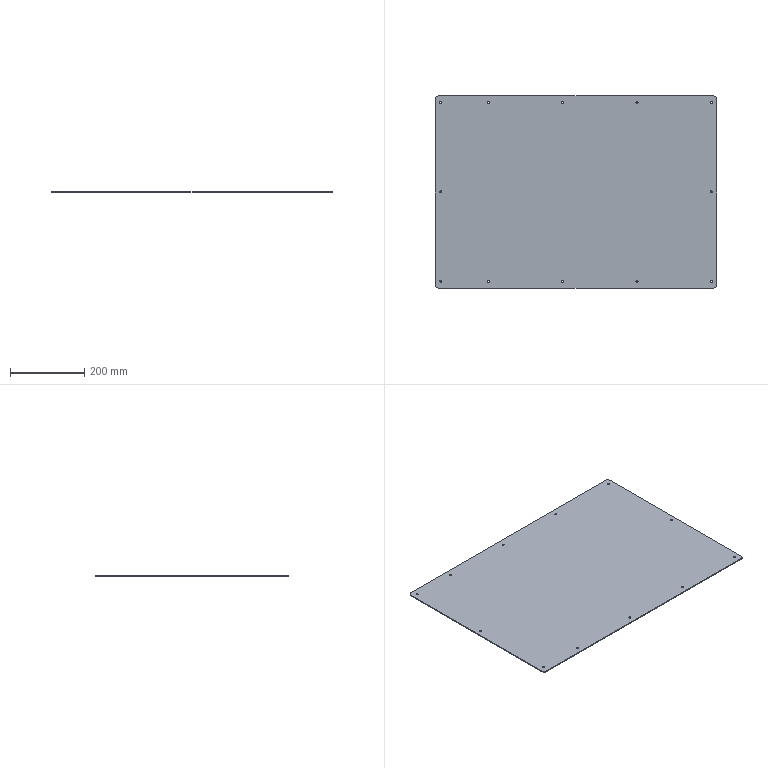Part | STEP file | MT-COMBO-119-S008 | 1 solid | 34 faces | box 758 x 516.5 x 2.5 mm | volume 977840 mm3 | cylinder 28 | plane 6 | commonest cylinder face diameters 5.5 x24 20 x4
STEP:
#1=CARTESIAN_POINT('',(-33.25,240.25,2.5));
#2=VERTEX_POINT('',#1);
#3=CARTESIAN_POINT('',(-38.75,240.25,2.5));
#4=VERTEX_POINT('',#3);
#5=CARTESIAN_POINT('',(-36.,240.25,2.5));
#6=DIRECTION('',(0.,0.,-1.));
#7=DIRECTION('',(-1.,0.,0.));
#8=AXIS2_PLACEMENT_3D('',#5,#6,#7);
#9=CIRCLE('',#8,2.75);
#10=EDGE_CURVE('',#2,#4,#9,.T.);
#11=ORIENTED_EDGE('',*,*,#10,.F.);
#12=CARTESIAN_POINT('',(-33.25,240.25,0.));
#13=VERTEX_POINT('',#12);
#14=CARTESIAN_POINT('',(-33.25,240.25,0.));
#15=DIRECTION('',(0.,0.,-1.));
#16=VECTOR('',#15,1000.);
#17=LINE('',#14,#16);
#18=EDGE_CURVE('',#2,#13,#17,.T.);
#19=ORIENTED_EDGE('',*,*,#18,.T.);
#20=CARTESIAN_POINT('',(-38.75,240.25,0.));
#21=VERTEX_POINT('',#20);
#22=CARTESIAN_POINT('',(-36.,240.25,0.));
#23=DIRECTION('',(0.,0.,-1.));
#24=DIRECTION('',(-1.,0.,0.));
#25=AXIS2_PLACEMENT_3D('',#22,#23,#24);
#26=CIRCLE('',#25,2.75);
#27=EDGE_CURVE('',#13,#21,#26,.T.);
#28=ORIENTED_EDGE('',*,*,#27,.T.);
#29=CARTESIAN_POINT('',(-38.75,240.25,0.));
#30=DIRECTION('',(0.,0.,-1.));
#31=VECTOR('',#30,1000.);
#32=LINE('',#29,#31);
#33=EDGE_CURVE('',#4,#21,#32,.T.);
#34=ORIENTED_EDGE('',*,*,#33,.F.);
#35=EDGE_LOOP('',(#11,#19,#28,#34));
#36=FACE_OUTER_BOUND('',#35,.T.);
#37=CARTESIAN_POINT('',(-36.,240.25,0.));
#38=DIRECTION('',(0.,0.,-1.));
#39=DIRECTION('',(-1.,0.,0.));
#40=AXIS2_PLACEMENT_3D('',#37,#38,#39);
#41=CYLINDRICAL_SURFACE('',#40,2.75);
#42=ADVANCED_FACE('',(#36),#41,.F.);
#43=CARTESIAN_POINT('',(-233.25,-240.25,2.5));
#44=VERTEX_POINT('',#43);
#45=CARTESIAN_POINT('',(-238.75,-240.25,2.5));
#46=VERTEX_POINT('',#45);
#47=CARTESIAN_POINT('',(-236.,-240.25,2.5));
#48=DIRECTION('',(0.,0.,-1.));
#49=DIRECTION('',(-1.,0.,0.));
#50=AXIS2_PLACEMENT_3D('',#47,#48,#49);
#51=CIRCLE('',#50,2.75);
#52=EDGE_CURVE('',#44,#46,#51,.T.);
#53=ORIENTED_EDGE('',*,*,#52,.F.);
#54=CARTESIAN_POINT('',(-233.25,-240.25,0.));
#55=VERTEX_POINT('',#54);
#56=CARTESIAN_POINT('',(-233.25,-240.25,0.));
#57=DIRECTION('',(0.,0.,-1.));
#58=VECTOR('',#57,1000.);
#59=LINE('',#56,#58);
#60=EDGE_CURVE('',#44,#55,#59,.T.);
#61=ORIENTED_EDGE('',*,*,#60,.T.);
#62=CARTESIAN_POINT('',(-238.75,-240.25,0.));
#63=VERTEX_POINT('',#62);
#64=CARTESIAN_POINT('',(-236.,-240.25,0.));
#65=DIRECTION('',(0.,0.,-1.));
#66=DIRECTION('',(-1.,0.,0.));
#67=AXIS2_PLACEMENT_3D('',#64,#65,#66);
#68=CIRCLE('',#67,2.75);
#69=EDGE_CURVE('',#55,#63,#68,.T.);
#70=ORIENTED_EDGE('',*,*,#69,.T.);
#71=CARTESIAN_POINT('',(-238.75,-240.25,0.));
#72=DIRECTION('',(0.,0.,-1.));
#73=VECTOR('',#72,1000.);
#74=LINE('',#71,#73);
#75=EDGE_CURVE('',#46,#63,#74,.T.);
#76=ORIENTED_EDGE('',*,*,#75,.F.);
#77=EDGE_LOOP('',(#53,#61,#70,#76));
#78=FACE_OUTER_BOUND('',#77,.T.);
#79=CARTESIAN_POINT('',(-236.,-240.25,0.));
#80=DIRECTION('',(0.,0.,-1.));
#81=DIRECTION('',(-1.,0.,0.));
#82=AXIS2_PLACEMENT_3D('',#79,#80,#81);
#83=CYLINDRICAL_SURFACE('',#82,2.75);
#84=ADVANCED_FACE('',(#78),#83,.F.);
#85=CARTESIAN_POINT('',(-33.25,-240.25,2.5));
#86=VERTEX_POINT('',#85);
#87=CARTESIAN_POINT('',(-38.75,-240.25,2.5));
#88=VERTEX_POINT('',#87);
#89=CARTESIAN_POINT('',(-36.,-240.25,2.5));
#90=DIRECTION('',(0.,0.,-1.));
#91=DIRECTION('',(-1.,0.,0.));
#92=AXIS2_PLACEMENT_3D('',#89,#90,#91);
#93=CIRCLE('',#92,2.75);
#94=EDGE_CURVE('',#86,#88,#93,.T.);
#95=ORIENTED_EDGE('',*,*,#94,.F.);
#96=CARTESIAN_POINT('',(-33.25,-240.25,0.));
#97=VERTEX_POINT('',#96);
#98=CARTESIAN_POINT('',(-33.25,-240.25,0.));
#99=DIRECTION('',(0.,0.,-1.));
#100=VECTOR('',#99,1000.);
#101=LINE('',#98,#100);
#102=EDGE_CURVE('',#86,#97,#101,.T.);
#103=ORIENTED_EDGE('',*,*,#102,.T.);
#104=CARTESIAN_POINT('',(-38.75,-240.25,0.));
#105=VERTEX_POINT('',#104);
#106=CARTESIAN_POINT('',(-36.,-240.25,0.));
#107=DIRECTION('',(0.,0.,-1.));
#108=DIRECTION('',(-1.,0.,0.));
#109=AXIS2_PLACEMENT_3D('',#106,#107,#108);
#110=CIRCLE('',#109,2.75);
#111=EDGE_CURVE('',#97,#105,#110,.T.);
#112=ORIENTED_EDGE('',*,*,#111,.T.);
#113=CARTESIAN_POINT('',(-38.75,-240.25,0.));
#114=DIRECTION('',(0.,0.,-1.));
#115=VECTOR('',#114,1000.);
#116=LINE('',#113,#115);
#117=EDGE_CURVE('',#88,#105,#116,.T.);
#118=ORIENTED_EDGE('',*,*,#117,.F.);
#119=EDGE_LOOP('',(#95,#103,#112,#118));
#120=FACE_OUTER_BOUND('',#119,.T.);
#121=CARTESIAN_POINT('',(-36.,-240.25,0.));
#122=DIRECTION('',(0.,0.,-1.));
#123=DIRECTION('',(-1.,0.,0.));
#124=AXIS2_PLACEMENT_3D('',#121,#122,#123);
#125=CYLINDRICAL_SURFACE('',#124,2.75);
#126=ADVANCED_FACE('',(#120),#125,.F.);
#127=CARTESIAN_POINT('',(166.75,-240.25,2.5));
#128=VERTEX_POINT('',#127);
#129=CARTESIAN_POINT('',(161.25,-240.25,2.5));
#130=VERTEX_POINT('',#129);
#131=CARTESIAN_POINT('',(164.,-240.25,2.5));
#132=DIRECTION('',(0.,0.,-1.));
#133=DIRECTION('',(-1.,0.,0.));
#134=AXIS2_PLACEMENT_3D('',#131,#132,#133);
#135=CIRCLE('',#134,2.75);
#136=EDGE_CURVE('',#128,#130,#135,.T.);
#137=ORIENTED_EDGE('',*,*,#136,.F.);
#138=CARTESIAN_POINT('',(166.75,-240.25,0.));
#139=VERTEX_POINT('',#138);
#140=CARTESIAN_POINT('',(166.75,-240.25,0.));
#141=DIRECTION('',(0.,0.,-1.));
#142=VECTOR('',#141,1000.);
#143=LINE('',#140,#142);
#144=EDGE_CURVE('',#128,#139,#143,.T.);
#145=ORIENTED_EDGE('',*,*,#144,.T.);
#146=CARTESIAN_POINT('',(161.25,-240.25,0.));
#147=VERTEX_POINT('',#146);
#148=CARTESIAN_POINT('',(164.,-240.25,0.));
#149=DIRECTION('',(0.,0.,-1.));
#150=DIRECTION('',(-1.,0.,0.));
#151=AXIS2_PLACEMENT_3D('',#148,#149,#150);
#152=CIRCLE('',#151,2.75);
#153=EDGE_CURVE('',#139,#147,#152,.T.);
#154=ORIENTED_EDGE('',*,*,#153,.T.);
#155=CARTESIAN_POINT('',(161.25,-240.25,0.));
#156=DIRECTION('',(0.,0.,-1.));
#157=VECTOR('',#156,1000.);
#158=LINE('',#155,#157);
#159=EDGE_CURVE('',#130,#147,#158,.T.);
#160=ORIENTED_EDGE('',*,*,#159,.F.);
#161=EDGE_LOOP('',(#137,#145,#154,#160));
#162=FACE_OUTER_BOUND('',#161,.T.);
#163=CARTESIAN_POINT('',(164.,-240.25,0.));
#164=DIRECTION('',(0.,0.,-1.));
#165=DIRECTION('',(-1.,0.,0.));
#166=AXIS2_PLACEMENT_3D('',#163,#164,#165);
#167=CYLINDRICAL_SURFACE('',#166,2.75);
#168=ADVANCED_FACE('',(#162),#167,.F.);
#169=CARTESIAN_POINT('',(366.75,240.25,2.5));
#170=VERTEX_POINT('',#169);
#171=CARTESIAN_POINT('',(361.25,240.25,2.5));
#172=VERTEX_POINT('',#171);
#173=CARTESIAN_POINT('',(364.,240.25,2.5));
#174=DIRECTION('',(0.,0.,-1.));
#175=DIRECTION('',(-1.,0.,0.));
#176=AXIS2_PLACEMENT_3D('',#173,#174,#175);
#177=CIRCLE('',#176,2.75);
#178=EDGE_CURVE('',#170,#172,#177,.T.);
#179=ORIENTED_EDGE('',*,*,#178,.F.);
#180=CARTESIAN_POINT('',(366.75,240.25,0.));
#181=VERTEX_POINT('',#180);
#182=CARTESIAN_POINT('',(366.75,240.25,0.));
#183=DIRECTION('',(0.,0.,-1.));
#184=VECTOR('',#183,1000.);
#185=LINE('',#182,#184);
#186=EDGE_CURVE('',#170,#181,#185,.T.);
#187=ORIENTED_EDGE('',*,*,#186,.T.);
#188=CARTESIAN_POINT('',(361.25,240.25,0.));
#189=VERTEX_POINT('',#188);
#190=CARTESIAN_POINT('',(364.,240.25,0.));
#191=DIRECTION('',(0.,0.,-1.));
#192=DIRECTION('',(-1.,0.,0.));
#193=AXIS2_PLACEMENT_3D('',#190,#191,#192);
#194=CIRCLE('',#193,2.75);
#195=EDGE_CURVE('',#181,#189,#194,.T.);
#196=ORIENTED_EDGE('',*,*,#195,.T.);
#197=CARTESIAN_POINT('',(361.25,240.25,0.));
#198=DIRECTION('',(0.,0.,-1.));
#199=VECTOR('',#198,1000.);
#200=LINE('',#197,#199);
#201=EDGE_CURVE('',#172,#189,#200,.T.);
#202=ORIENTED_EDGE('',*,*,#201,.F.);
#203=EDGE_LOOP('',(#179,#187,#196,#202));
#204=FACE_OUTER_BOUND('',#203,.T.);
#205=CARTESIAN_POINT('',(364.,240.25,0.));
#206=DIRECTION('',(0.,0.,-1.));
#207=DIRECTION('',(-1.,0.,0.));
#208=AXIS2_PLACEMENT_3D('',#205,#206,#207);
#209=CYLINDRICAL_SURFACE('',#208,2.75);
#210=ADVANCED_FACE('',(#204),#209,.F.);
#211=CARTESIAN_POINT('',(366.75,-240.25,2.5));
#212=VERTEX_POINT('',#211);
#213=CARTESIAN_POINT('',(361.25,-240.25,2.5));
#214=VERTEX_POINT('',#213);
#215=CARTESIAN_POINT('',(364.,-240.25,2.5));
#216=DIRECTION('',(0.,0.,-1.));
#217=DIRECTION('',(-1.,0.,0.));
#218=AXIS2_PLACEMENT_3D('',#215,#216,#217);
#219=CIRCLE('',#218,2.75);
#220=EDGE_CURVE('',#212,#214,#219,.T.);
#221=ORIENTED_EDGE('',*,*,#220,.F.);
#222=CARTESIAN_POINT('',(366.75,-240.25,0.));
#223=VERTEX_POINT('',#222);
#224=CARTESIAN_POINT('',(366.75,-240.25,0.));
#225=DIRECTION('',(0.,0.,-1.));
#226=VECTOR('',#225,1000.);
#227=LINE('',#224,#226);
#228=EDGE_CURVE('',#212,#223,#227,.T.);
#229=ORIENTED_EDGE('',*,*,#228,.T.);
#230=CARTESIAN_POINT('',(361.25,-240.25,0.));
#231=VERTEX_POINT('',#230);
#232=CARTESIAN_POINT('',(364.,-240.25,0.));
#233=DIRECTION('',(0.,0.,-1.));
#234=DIRECTION('',(-1.,0.,0.));
#235=AXIS2_PLACEMENT_3D('',#232,#233,#234);
#236=CIRCLE('',#235,2.75);
#237=EDGE_CURVE('',#223,#231,#236,.T.);
#238=ORIENTED_EDGE('',*,*,#237,.T.);
#239=CARTESIAN_POINT('',(361.25,-240.25,0.));
#240=DIRECTION('',(0.,0.,-1.));
#241=VECTOR('',#240,1000.);
#242=LINE('',#239,#241);
#243=EDGE_CURVE('',#214,#231,#242,.T.);
#244=ORIENTED_EDGE('',*,*,#243,.F.);
#245=EDGE_LOOP('',(#221,#229,#238,#244));
#246=FACE_OUTER_BOUND('',#245,.T.);
#247=CARTESIAN_POINT('',(364.,-240.25,0.));
#248=DIRECTION('',(0.,0.,-1.));
#249=DIRECTION('',(-1.,0.,0.));
#250=AXIS2_PLACEMENT_3D('',#247,#248,#249);
#251=CYLINDRICAL_SURFACE('',#250,2.75);
#252=ADVANCED_FACE('',(#246),#251,.F.);
#253=CARTESIAN_POINT('',(366.75,0.25,2.5));
#254=VERTEX_POINT('',#253);
#255=CARTESIAN_POINT('',(361.25,0.25,2.5));
#256=VERTEX_POINT('',#255);
#257=CARTESIAN_POINT('',(364.,0.25,2.5));
#258=DIRECTION('',(0.,0.,-1.));
#259=DIRECTION('',(-1.,0.,0.));
#260=AXIS2_PLACEMENT_3D('',#257,#258,#259);
#261=CIRCLE('',#260,2.75);
#262=EDGE_CURVE('',#254,#256,#261,.T.);
#263=ORIENTED_EDGE('',*,*,#262,.F.);
#264=CARTESIAN_POINT('',(366.75,0.25,0.));
#265=VERTEX_POINT('',#264);
#266=CARTESIAN_POINT('',(366.75,0.25,0.));
#267=DIRECTION('',(0.,0.,-1.));
#268=VECTOR('',#267,1000.);
#269=LINE('',#266,#268);
#270=EDGE_CURVE('',#254,#265,#269,.T.);
#271=ORIENTED_EDGE('',*,*,#270,.T.);
#272=CARTESIAN_POINT('',(361.25,0.25,0.));
#273=VERTEX_POINT('',#272);
#274=CARTESIAN_POINT('',(364.,0.25,0.));
#275=DIRECTION('',(0.,0.,-1.));
#276=DIRECTION('',(-1.,0.,0.));
#277=AXIS2_PLACEMENT_3D('',#274,#275,#276);
#278=CIRCLE('',#277,2.75);
#279=EDGE_CURVE('',#265,#273,#278,.T.);
#280=ORIENTED_EDGE('',*,*,#279,.T.);
#281=CARTESIAN_POINT('',(361.25,0.25,0.));
#282=DIRECTION('',(0.,0.,-1.));
#283=VECTOR('',#282,1000.);
#284=LINE('',#281,#283);
#285=EDGE_CURVE('',#256,#273,#284,.T.);
#286=ORIENTED_EDGE('',*,*,#285,.F.);
#287=EDGE_LOOP('',(#263,#271,#280,#286));
#288=FACE_OUTER_BOUND('',#287,.T.);
#289=CARTESIAN_POINT('',(364.,0.25,0.));
#290=DIRECTION('',(0.,0.,-1.));
#291=DIRECTION('',(-1.,0.,0.));
#292=AXIS2_PLACEMENT_3D('',#289,#290,#291);
#293=CYLINDRICAL_SURFACE('',#292,2.75);
#294=ADVANCED_FACE('',(#288),#293,.F.);
#295=CARTESIAN_POINT('',(-361.25,240.25,2.5));
#296=VERTEX_POINT('',#295);
#297=CARTESIAN_POINT('',(-366.75,240.25,2.5));
#298=VERTEX_POINT('',#297);
#299=CARTESIAN_POINT('',(-364.,240.25,2.5));
#300=DIRECTION('',(0.,0.,-1.));
#301=DIRECTION('',(-1.,0.,0.));
#302=AXIS2_PLACEMENT_3D('',#299,#300,#301);
#303=CIRCLE('',#302,2.75);
#304=EDGE_CURVE('',#296,#298,#303,.T.);
#305=ORIENTED_EDGE('',*,*,#304,.F.);
#306=CARTESIAN_POINT('',(-361.25,240.25,0.));
#307=VERTEX_POINT('',#306);
#308=CARTESIAN_POINT('',(-361.25,240.25,0.));
#309=DIRECTION('',(0.,0.,-1.));
#310=VECTOR('',#309,1000.);
#311=LINE('',#308,#310);
#312=EDGE_CURVE('',#296,#307,#311,.T.);
#313=ORIENTED_EDGE('',*,*,#312,.T.);
#314=CARTESIAN_POINT('',(-366.75,240.25,0.));
#315=VERTEX_POINT('',#314);
#316=CARTESIAN_POINT('',(-364.,240.25,0.));
#317=DIRECTION('',(0.,0.,-1.));
#318=DIRECTION('',(-1.,0.,0.));
#319=AXIS2_PLACEMENT_3D('',#316,#317,#318);
#320=CIRCLE('',#319,2.75);
#321=EDGE_CURVE('',#307,#315,#320,.T.);
#322=ORIENTED_EDGE('',*,*,#321,.T.);
#323=CARTESIAN_POINT('',(-366.75,240.25,0.));
#324=DIRECTION('',(0.,0.,-1.));
#325=VECTOR('',#324,1000.);
#326=LINE('',#323,#325);
#327=EDGE_CURVE('',#298,#315,#326,.T.);
#328=ORIENTED_EDGE('',*,*,#327,.F.);
#329=EDGE_LOOP('',(#305,#313,#322,#328));
#330=FACE_OUTER_BOUND('',#329,.T.);
#331=CARTESIAN_POINT('',(-364.,240.25,0.));
#332=DIRECTION('',(0.,0.,-1.));
#333=DIRECTION('',(-1.,0.,0.));
#334=AXIS2_PLACEMENT_3D('',#331,#332,#333);
#335=CYLINDRICAL_SURFACE('',#334,2.75);
#336=ADVANCED_FACE('',(#330),#335,.F.);
#337=CARTESIAN_POINT('',(-361.25,-239.75,2.5));
#338=VERTEX_POINT('',#337);
#339=CARTESIAN_POINT('',(-366.75,-239.75,2.5));
#340=VERTEX_POINT('',#339);
#341=CARTESIAN_POINT('',(-364.,-239.75,2.5));
#342=DIRECTION('',(0.,0.,-1.));
#343=DIRECTION('',(-1.,0.,0.));
#344=AXIS2_PLACEMENT_3D('',#341,#342,#343);
#345=CIRCLE('',#344,2.75);
#346=EDGE_CURVE('',#338,#340,#345,.T.);
#347=ORIENTED_EDGE('',*,*,#346,.F.);
#348=CARTESIAN_POINT('',(-361.25,-239.75,0.));
#349=VERTEX_POINT('',#348);
#350=CARTESIAN_POINT('',(-361.25,-239.75,0.));
#351=DIRECTION('',(0.,0.,-1.));
#352=VECTOR('',#351,1000.);
#353=LINE('',#350,#352);
#354=EDGE_CURVE('',#338,#349,#353,.T.);
#355=ORIENTED_EDGE('',*,*,#354,.T.);
#356=CARTESIAN_POINT('',(-366.75,-239.75,0.));
#357=VERTEX_POINT('',#356);
#358=CARTESIAN_POINT('',(-364.,-239.75,0.));
#359=DIRECTION('',(0.,0.,-1.));
#360=DIRECTION('',(-1.,0.,0.));
#361=AXIS2_PLACEMENT_3D('',#358,#359,#360);
#362=CIRCLE('',#361,2.75);
#363=EDGE_CURVE('',#349,#357,#362,.T.);
#364=ORIENTED_EDGE('',*,*,#363,.T.);
#365=CARTESIAN_POINT('',(-366.75,-239.75,0.));
#366=DIRECTION('',(0.,0.,-1.));
#367=VECTOR('',#366,1000.);
#368=LINE('',#365,#367);
#369=EDGE_CURVE('',#340,#357,#368,.T.);
#370=ORIENTED_EDGE('',*,*,#369,.F.);
#371=EDGE_LOOP('',(#347,#355,#364,#370));
#372=FACE_OUTER_BOUND('',#371,.T.);
#373=CARTESIAN_POINT('',(-364.,-239.75,0.));
#374=DIRECTION('',(0.,0.,-1.));
#375=DIRECTION('',(-1.,0.,0.));
#376=AXIS2_PLACEMENT_3D('',#373,#374,#375);
#377=CYLINDRICAL_SURFACE('',#376,2.75);
#378=ADVANCED_FACE('',(#372),#377,.F.);
#379=CARTESIAN_POINT('',(-361.25,0.25,2.5));
#380=VERTEX_POINT('',#379);
#381=CARTESIAN_POINT('',(-366.75,0.25,2.5));
#382=VERTEX_POINT('',#381);
#383=CARTESIAN_POINT('',(-364.,0.25,2.5));
#384=DIRECTION('',(0.,0.,-1.));
#385=DIRECTION('',(-1.,0.,0.));
#386=AXIS2_PLACEMENT_3D('',#383,#384,#385);
#387=CIRCLE('',#386,2.75);
#388=EDGE_CURVE('',#380,#382,#387,.T.);
#389=ORIENTED_EDGE('',*,*,#388,.F.);
#390=CARTESIAN_POINT('',(-361.25,0.25,0.));
#391=VERTEX_POINT('',#390);
#392=CARTESIAN_POINT('',(-361.25,0.25,0.));
#393=DIRECTION('',(0.,0.,-1.));
#394=VECTOR('',#393,1000.);
#395=LINE('',#392,#394);
#396=EDGE_CURVE('',#380,#391,#395,.T.);
#397=ORIENTED_EDGE('',*,*,#396,.T.);
#398=CARTESIAN_POINT('',(-366.75,0.25,0.));
#399=VERTEX_POINT('',#398);
#400=CARTESIAN_POINT('',(-364.,0.25,0.));
#401=DIRECTION('',(0.,0.,-1.));
#402=DIRECTION('',(-1.,0.,0.));
#403=AXIS2_PLACEMENT_3D('',#400,#401,#402);
#404=CIRCLE('',#403,2.75);
#405=EDGE_CURVE('',#391,#399,#404,.T.);
#406=ORIENTED_EDGE('',*,*,#405,.T.);
#407=CARTESIAN_POINT('',(-366.75,0.25,0.));
#408=DIRECTION('',(0.,0.,-1.));
#409=VECTOR('',#408,1000.);
#410=LINE('',#407,#409);
#411=EDGE_CURVE('',#382,#399,#410,.T.);
#412=ORIENTED_EDGE('',*,*,#411,.F.);
#413=EDGE_LOOP('',(#389,#397,#406,#412));
#414=FACE_OUTER_BOUND('',#413,.T.);
#415=CARTESIAN_POINT('',(-364.,0.25,0.));
#416=DIRECTION('',(0.,0.,-1.));
#417=DIRECTION('',(-1.,0.,0.));
#418=AXIS2_PLACEMENT_3D('',#415,#416,#417);
#419=CYLINDRICAL_SURFACE('',#418,2.75);
#420=ADVANCED_FACE('',(#414),#419,.F.);
#421=CARTESIAN_POINT('',(166.75,240.25,2.5));
#422=VERTEX_POINT('',#421);
#423=CARTESIAN_POINT('',(161.25,240.25,2.5));
#424=VERTEX_POINT('',#423);
#425=CARTESIAN_POINT('',(164.,240.25,2.5));
#426=DIRECTION('',(0.,0.,-1.));
#427=DIRECTION('',(-1.,0.,0.));
#428=AXIS2_PLACEMENT_3D('',#425,#426,#427);
#429=CIRCLE('',#428,2.75);
#430=EDGE_CURVE('',#422,#424,#429,.T.);
#431=ORIENTED_EDGE('',*,*,#430,.F.);
#432=CARTESIAN_POINT('',(166.75,240.25,0.));
#433=VERTEX_POINT('',#432);
#434=CARTESIAN_POINT('',(166.75,240.25,0.));
#435=DIRECTION('',(0.,0.,-1.));
#436=VECTOR('',#435,1000.);
#437=LINE('',#434,#436);
#438=EDGE_CURVE('',#422,#433,#437,.T.);
#439=ORIENTED_EDGE('',*,*,#438,.T.);
#440=CARTESIAN_POINT('',(161.25,240.25,0.));
#441=VERTEX_POINT('',#440);
#442=CARTESIAN_POINT('',(164.,240.25,0.));
#443=DIRECTION('',(0.,0.,-1.));
#444=DIRECTION('',(-1.,0.,0.));
#445=AXIS2_PLACEMENT_3D('',#442,#443,#444);
#446=CIRCLE('',#445,2.75);
#447=EDGE_CURVE('',#433,#441,#446,.T.);
#448=ORIENTED_EDGE('',*,*,#447,.T.);
#449=CARTESIAN_POINT('',(161.25,240.25,0.));
#450=DIRECTION('',(0.,0.,-1.));
#451=VECTOR('',#450,1000.);
#452=LINE('',#449,#451);
#453=EDGE_CURVE('',#424,#441,#452,.T.);
#454=ORIENTED_EDGE('',*,*,#453,.F.);
#455=EDGE_LOOP('',(#431,#439,#448,#454));
#456=FACE_OUTER_BOUND('',#455,.T.);
#457=CARTESIAN_POINT('',(164.,240.25,0.));
#458=DIRECTION('',(0.,0.,-1.));
#459=DIRECTION('',(-1.,0.,0.));
#460=AXIS2_PLACEMENT_3D('',#457,#458,#459);
#461=CYLINDRICAL_SURFACE('',#460,2.75);
#462=ADVANCED_FACE('',(#456),#461,.F.);
#463=CARTESIAN_POINT('',(-233.25,240.25,2.5));
#464=VERTEX_POINT('',#463);
#465=CARTESIAN_POINT('',(-238.75,240.25,2.5));
#466=VERTEX_POINT('',#465);
#467=CARTESIAN_POINT('',(-236.,240.25,2.5));
#468=DIRECTION('',(0.,0.,-1.));
#469=DIRECTION('',(-1.,0.,0.));
#470=AXIS2_PLACEMENT_3D('',#467,#468,#469);
#471=CIRCLE('',#470,2.75);
#472=EDGE_CURVE('',#464,#466,#471,.T.);
#473=ORIENTED_EDGE('',*,*,#472,.F.);
#474=CARTESIAN_POINT('',(-233.25,240.25,0.));
#475=VERTEX_POINT('',#474);
#476=CARTESIAN_POINT('',(-233.25,240.25,0.));
#477=DIRECTION('',(0.,0.,-1.));
#478=VECTOR('',#477,1000.);
#479=LINE('',#476,#478);
#480=EDGE_CURVE('',#464,#475,#479,.T.);
#481=ORIENTED_EDGE('',*,*,#480,.T.);
#482=CARTESIAN_POINT('',(-238.75,240.25,0.));
#483=VERTEX_POINT('',#482);
#484=CARTESIAN_POINT('',(-236.,240.25,0.));
#485=DIRECTION('',(0.,0.,-1.));
#486=DIRECTION('',(-1.,0.,0.));
#487=AXIS2_PLACEMENT_3D('',#484,#485,#486);
#488=CIRCLE('',#487,2.75);
#489=EDGE_CURVE('',#475,#483,#488,.T.);
#490=ORIENTED_EDGE('',*,*,#489,.T.);
#491=CARTESIAN_POINT('',(-238.75,240.25,0.));
#492=DIRECTION('',(0.,0.,-1.));
#493=VECTOR('',#492,1000.);
#494=LINE('',#491,#493);
#495=EDGE_CURVE('',#466,#483,#494,.T.);
#496=ORIENTED_EDGE('',*,*,#495,.F.);
#497=EDGE_LOOP('',(#473,#481,#490,#496));
#498=FACE_OUTER_BOUND('',#497,.T.);
#499=CARTESIAN_POINT('',(-236.,240.25,0.));
#500=DIRECTION('',(0.,0.,-1.));
#501=DIRECTION('',(-1.,0.,0.));
#502=AXIS2_PLACEMENT_3D('',#499,#500,#501);
#503=CYLINDRICAL_SURFACE('',#502,2.75);
#504=ADVANCED_FACE('',(#498),#503,.F.);
#505=CARTESIAN_POINT('',(-36.,240.25,2.5));
#506=DIRECTION('',(0.,0.,-1.));
#507=DIRECTION('',(-1.,0.,0.));
#508=AXIS2_PLACEMENT_3D('',#505,#506,#507);
#509=CIRCLE('',#508,2.75);
#510=EDGE_CURVE('',#4,#2,#509,.T.);
#511=ORIENTED_EDGE('',*,*,#510,.T.);
#512=ORIENTED_EDGE('',*,*,#10,.T.);
#513=EDGE_LOOP('',(#511,#512));
#514=FACE_BOUND('',#513,.T.);
#515=CARTESIAN_POINT('',(-236.,-240.25,2.5));
#516=DIRECTION('',(0.,0.,-1.));
#517=DIRECTION('',(-1.,0.,0.));
#518=AXIS2_PLACEMENT_3D('',#515,#516,#517);
#519=CIRCLE('',#518,2.75);
#520=EDGE_CURVE('',#46,#44,#519,.T.);
#521=ORIENTED_EDGE('',*,*,#520,.T.);
#522=ORIENTED_EDGE('',*,*,#52,.T.);
#523=EDGE_LOOP('',(#521,#522));
#524=FACE_BOUND('',#523,.T.);
#525=CARTESIAN_POINT('',(-36.,-240.25,2.5));
#526=DIRECTION('',(0.,0.,-1.));
#527=DIRECTION('',(-1.,0.,0.));
#528=AXIS2_PLACEMENT_3D('',#525,#526,#527);
#529=CIRCLE('',#528,2.75);
#530=EDGE_CURVE('',#88,#86,#529,.T.);
#531=ORIENTED_EDGE('',*,*,#530,.T.);
#532=ORIENTED_EDGE('',*,*,#94,.T.);
#533=EDGE_LOOP('',(#531,#532));
#534=FACE_BOUND('',#533,.T.);
#535=CARTESIAN_POINT('',(164.,-240.25,2.5));
#536=DIRECTION('',(0.,0.,-1.));
#537=DIRECTION('',(-1.,0.,0.));
#538=AXIS2_PLACEMENT_3D('',#535,#536,#537);
#539=CIRCLE('',#538,2.75);
#540=EDGE_CURVE('',#130,#128,#539,.T.);
#541=ORIENTED_EDGE('',*,*,#540,.T.);
#542=ORIENTED_EDGE('',*,*,#136,.T.);
#543=EDGE_LOOP('',(#541,#542));
#544=FACE_BOUND('',#543,.T.);
#545=CARTESIAN_POINT('',(364.,240.25,2.5));
#546=DIRECTION('',(0.,0.,-1.));
#547=DIRECTION('',(-1.,0.,0.));
#548=AXIS2_PLACEMENT_3D('',#545,#546,#547);
#549=CIRCLE('',#548,2.75);
#550=EDGE_CURVE('',#172,#170,#549,.T.);
#551=ORIENTED_EDGE('',*,*,#550,.T.);
#552=ORIENTED_EDGE('',*,*,#178,.T.);
#553=EDGE_LOOP('',(#551,#552));
#554=FACE_BOUND('',#553,.T.);
#555=CARTESIAN_POINT('',(364.,-240.25,2.5));
#556=DIRECTION('',(0.,0.,-1.));
#557=DIRECTION('',(-1.,0.,0.));
#558=AXIS2_PLACEMENT_3D('',#555,#556,#557);
#559=CIRCLE('',#558,2.75);
#560=EDGE_CURVE('',#214,#212,#559,.T.);
#561=ORIENTED_EDGE('',*,*,#560,.T.);
#562=ORIENTED_EDGE('',*,*,#220,.T.);
#563=EDGE_LOOP('',(#561,#562));
#564=FACE_BOUND('',#563,.T.);
#565=CARTESIAN_POINT('',(-379.,248.25,2.5));
#566=VERTEX_POINT('',#565);
#567=CARTESIAN_POINT('',(-379.,-248.25,2.5));
#568=VERTEX_POINT('',#567);
#569=CARTESIAN_POINT('',(-379.,-258.25,2.5));
#570=DIRECTION('',(0.,-1.,0.));
#571=VECTOR('',#570,1000.);
#572=LINE('',#569,#571);
#573=EDGE_CURVE('',#566,#568,#572,.T.);
#574=ORIENTED_EDGE('',*,*,#573,.T.);
#575=CARTESIAN_POINT('',(-369.,-258.25,2.5));
#576=VERTEX_POINT('',#575);
#577=CARTESIAN_POINT('',(-369.,-248.25,2.5));
#578=DIRECTION('',(0.,0.,1.));
#579=DIRECTION('',(1.,0.,0.));
#580=AXIS2_PLACEMENT_3D('',#577,#578,#579);
#581=CIRCLE('',#580,10.);
#582=EDGE_CURVE('',#568,#576,#581,.T.);
#583=ORIENTED_EDGE('',*,*,#582,.T.);
#584=CARTESIAN_POINT('',(369.,-258.25,2.5));
#585=VERTEX_POINT('',#584);
#586=CARTESIAN_POINT('',(379.,-258.25,2.5));
#587=DIRECTION('',(1.,0.,0.));
#588=VECTOR('',#587,1000.);
#589=LINE('',#586,#588);
#590=EDGE_CURVE('',#576,#585,#589,.T.);
#591=ORIENTED_EDGE('',*,*,#590,.T.);
#592=CARTESIAN_POINT('',(379.,-248.25,2.5));
#593=VERTEX_POINT('',#592);
#594=CARTESIAN_POINT('',(369.,-248.25,2.5));
#595=DIRECTION('',(0.,0.,1.));
#596=DIRECTION('',(1.,0.,0.));
#597=AXIS2_PLACEMENT_3D('',#594,#595,#596);
#598=CIRCLE('',#597,10.);
#599=EDGE_CURVE('',#585,#593,#598,.T.);
#600=ORIENTED_EDGE('',*,*,#599,.T.);
#601=CARTESIAN_POINT('',(379.,248.25,2.5));
#602=VERTEX_POINT('',#601);
#603=CARTESIAN_POINT('',(379.,-258.25,2.5));
#604=DIRECTION('',(0.,1.,0.));
#605=VECTOR('',#604,1000.);
#606=LINE('',#603,#605);
#607=EDGE_CURVE('',#593,#602,#606,.T.);
#608=ORIENTED_EDGE('',*,*,#607,.T.);
#609=CARTESIAN_POINT('',(369.,258.25,2.5));
#610=VERTEX_POINT('',#609);
#611=CARTESIAN_POINT('',(369.,248.25,2.5));
#612=DIRECTION('',(0.,0.,1.));
#613=DIRECTION('',(1.,0.,0.));
#614=AXIS2_PLACEMENT_3D('',#611,#612,#613);
#615=CIRCLE('',#614,10.);
#616=EDGE_CURVE('',#602,#610,#615,.T.);
#617=ORIENTED_EDGE('',*,*,#616,.T.);
#618=CARTESIAN_POINT('',(-369.,258.25,2.5));
#619=VERTEX_POINT('',#618);
#620=CARTESIAN_POINT('',(379.,258.25,2.5));
#621=DIRECTION('',(-1.,0.,0.));
#622=VECTOR('',#621,1000.);
#623=LINE('',#620,#622);
#624=EDGE_CURVE('',#610,#619,#623,.T.);
#625=ORIENTED_EDGE('',*,*,#624,.T.);
#626=CARTESIAN_POINT('',(-369.,248.25,2.5));
#627=DIRECTION('',(0.,0.,1.));
#628=DIRECTION('',(1.,0.,0.));
#629=AXIS2_PLACEMENT_3D('',#626,#627,#628);
#630=CIRCLE('',#629,10.);
#631=EDGE_CURVE('',#619,#566,#630,.T.);
#632=ORIENTED_EDGE('',*,*,#631,.T.);
#633=EDGE_LOOP('',(#574,#583,#591,#600,#608,#617,#625,#632));
#634=FACE_OUTER_BOUND('',#633,.T.);
#635=CARTESIAN_POINT('',(-236.,240.25,2.5));
#636=DIRECTION('',(0.,0.,-1.));
#637=DIRECTION('',(-1.,0.,0.));
#638=AXIS2_PLACEMENT_3D('',#635,#636,#637);
#639=CIRCLE('',#638,2.75);
#640=EDGE_CURVE('',#466,#464,#639,.T.);
#641=ORIENTED_EDGE('',*,*,#640,.T.);
#642=ORIENTED_EDGE('',*,*,#472,.T.);
#643=EDGE_LOOP('',(#641,#642));
#644=FACE_BOUND('',#643,.T.);
#645=CARTESIAN_POINT('',(164.,240.25,2.5));
#646=DIRECTION('',(0.,0.,-1.));
#647=DIRECTION('',(-1.,0.,0.));
#648=AXIS2_PLACEMENT_3D('',#645,#646,#647);
#649=CIRCLE('',#648,2.75);
#650=EDGE_CURVE('',#424,#422,#649,.T.);
#651=ORIENTED_EDGE('',*,*,#650,.T.);
#652=ORIENTED_EDGE('',*,*,#430,.T.);
#653=EDGE_LOOP('',(#651,#652));
#654=FACE_BOUND('',#653,.T.);
#655=CARTESIAN_POINT('',(-364.,0.25,2.5));
#656=DIRECTION('',(0.,0.,-1.));
#657=DIRECTION('',(-1.,0.,0.));
#658=AXIS2_PLACEMENT_3D('',#655,#656,#657);
#659=CIRCLE('',#658,2.75);
#660=EDGE_CURVE('',#382,#380,#659,.T.);
#661=ORIENTED_EDGE('',*,*,#660,.T.);
#662=ORIENTED_EDGE('',*,*,#388,.T.);
#663=EDGE_LOOP('',(#661,#662));
#664=FACE_BOUND('',#663,.T.);
#665=CARTESIAN_POINT('',(-364.,-239.75,2.5));
#666=DIRECTION('',(0.,0.,-1.));
#667=DIRECTION('',(-1.,0.,0.));
#668=AXIS2_PLACEMENT_3D('',#665,#666,#667);
#669=CIRCLE('',#668,2.75);
#670=EDGE_CURVE('',#340,#338,#669,.T.);
#671=ORIENTED_EDGE('',*,*,#670,.T.);
#672=ORIENTED_EDGE('',*,*,#346,.T.);
#673=EDGE_LOOP('',(#671,#672));
#674=FACE_BOUND('',#673,.T.);
#675=CARTESIAN_POINT('',(-364.,240.25,2.5));
#676=DIRECTION('',(0.,0.,-1.));
#677=DIRECTION('',(-1.,0.,0.));
#678=AXIS2_PLACEMENT_3D('',#675,#676,#677);
#679=CIRCLE('',#678,2.75);
#680=EDGE_CURVE('',#298,#296,#679,.T.);
#681=ORIENTED_EDGE('',*,*,#680,.T.);
#682=ORIENTED_EDGE('',*,*,#304,.T.);
#683=EDGE_LOOP('',(#681,#682));
#684=FACE_BOUND('',#683,.T.);
#685=CARTESIAN_POINT('',(364.,0.25,2.5));
#686=DIRECTION('',(0.,0.,-1.));
#687=DIRECTION('',(-1.,0.,0.));
#688=AXIS2_PLACEMENT_3D('',#685,#686,#687);
#689=CIRCLE('',#688,2.75);
#690=EDGE_CURVE('',#256,#254,#689,.T.);
#691=ORIENTED_EDGE('',*,*,#690,.T.);
#692=ORIENTED_EDGE('',*,*,#262,.T.);
#693=EDGE_LOOP('',(#691,#692));
#694=FACE_BOUND('',#693,.T.);
#695=CARTESIAN_POINT('',(0.,0.,2.5));
#696=DIRECTION('',(0.,0.,1.));
#697=DIRECTION('',(1.,0.,0.));
#698=AXIS2_PLACEMENT_3D('',#695,#696,#697);
#699=PLANE('',#698);
#700=ADVANCED_FACE('',(#514,#524,#534,#544,#554,#564,#634,#644,#654,#664,#674,#684,#694),#699,.T.);
#701=CARTESIAN_POINT('',(-36.,240.25,0.));
#702=DIRECTION('',(0.,0.,-1.));
#703=DIRECTION('',(-1.,0.,0.));
#704=AXIS2_PLACEMENT_3D('',#701,#702,#703);
#705=CIRCLE('',#704,2.75);
#706=EDGE_CURVE('',#21,#13,#705,.T.);
#707=ORIENTED_EDGE('',*,*,#706,.F.);
#708=ORIENTED_EDGE('',*,*,#27,.F.);
#709=EDGE_LOOP('',(#707,#708));
#710=FACE_BOUND('',#709,.T.);
#711=CARTESIAN_POINT('',(-236.,-240.25,0.));
#712=DIRECTION('',(0.,0.,-1.));
#713=DIRECTION('',(-1.,0.,0.));
#714=AXIS2_PLACEMENT_3D('',#711,#712,#713);
#715=CIRCLE('',#714,2.75);
#716=EDGE_CURVE('',#63,#55,#715,.T.);
#717=ORIENTED_EDGE('',*,*,#716,.F.);
#718=ORIENTED_EDGE('',*,*,#69,.F.);
#719=EDGE_LOOP('',(#717,#718));
#720=FACE_BOUND('',#719,.T.);
#721=CARTESIAN_POINT('',(-36.,-240.25,0.));
#722=DIRECTION('',(0.,0.,-1.));
#723=DIRECTION('',(-1.,0.,0.));
#724=AXIS2_PLACEMENT_3D('',#721,#722,#723);
#725=CIRCLE('',#724,2.75);
#726=EDGE_CURVE('',#105,#97,#725,.T.);
#727=ORIENTED_EDGE('',*,*,#726,.F.);
#728=ORIENTED_EDGE('',*,*,#111,.F.);
#729=EDGE_LOOP('',(#727,#728));
#730=FACE_BOUND('',#729,.T.);
#731=CARTESIAN_POINT('',(164.,-240.25,0.));
#732=DIRECTION('',(0.,0.,-1.));
#733=DIRECTION('',(-1.,0.,0.));
#734=AXIS2_PLACEMENT_3D('',#731,#732,#733);
#735=CIRCLE('',#734,2.75);
#736=EDGE_CURVE('',#147,#139,#735,.T.);
#737=ORIENTED_EDGE('',*,*,#736,.F.);
#738=ORIENTED_EDGE('',*,*,#153,.F.);
#739=EDGE_LOOP('',(#737,#738));
#740=FACE_BOUND('',#739,.T.);
#741=CARTESIAN_POINT('',(364.,240.25,0.));
#742=DIRECTION('',(0.,0.,-1.));
#743=DIRECTION('',(-1.,0.,0.));
#744=AXIS2_PLACEMENT_3D('',#741,#742,#743);
#745=CIRCLE('',#744,2.75);
#746=EDGE_CURVE('',#189,#181,#745,.T.);
#747=ORIENTED_EDGE('',*,*,#746,.F.);
#748=ORIENTED_EDGE('',*,*,#195,.F.);
#749=EDGE_LOOP('',(#747,#748));
#750=FACE_BOUND('',#749,.T.);
#751=CARTESIAN_POINT('',(364.,-240.25,0.));
#752=DIRECTION('',(0.,0.,-1.));
#753=DIRECTION('',(-1.,0.,0.));
#754=AXIS2_PLACEMENT_3D('',#751,#752,#753);
#755=CIRCLE('',#754,2.75);
#756=EDGE_CURVE('',#231,#223,#755,.T.);
#757=ORIENTED_EDGE('',*,*,#756,.F.);
#758=ORIENTED_EDGE('',*,*,#237,.F.);
#759=EDGE_LOOP('',(#757,#758));
#760=FACE_BOUND('',#759,.T.);
#761=CARTESIAN_POINT('',(364.,0.25,0.));
#762=DIRECTION('',(0.,0.,-1.));
#763=DIRECTION('',(-1.,0.,0.));
#764=AXIS2_PLACEMENT_3D('',#761,#762,#763);
#765=CIRCLE('',#764,2.75);
#766=EDGE_CURVE('',#273,#265,#765,.T.);
#767=ORIENTED_EDGE('',*,*,#766,.F.);
#768=ORIENTED_EDGE('',*,*,#279,.F.);
#769=EDGE_LOOP('',(#767,#768));
#770=FACE_BOUND('',#769,.T.);
#771=CARTESIAN_POINT('',(-364.,240.25,0.));
#772=DIRECTION('',(0.,0.,-1.));
#773=DIRECTION('',(-1.,0.,0.));
#774=AXIS2_PLACEMENT_3D('',#771,#772,#773);
#775=CIRCLE('',#774,2.75);
#776=EDGE_CURVE('',#315,#307,#775,.T.);
#777=ORIENTED_EDGE('',*,*,#776,.F.);
#778=ORIENTED_EDGE('',*,*,#321,.F.);
#779=EDGE_LOOP('',(#777,#778));
#780=FACE_BOUND('',#779,.T.);
#781=CARTESIAN_POINT('',(-364.,-239.75,0.));
#782=DIRECTION('',(0.,0.,-1.));
#783=DIRECTION('',(-1.,0.,0.));
#784=AXIS2_PLACEMENT_3D('',#781,#782,#783);
#785=CIRCLE('',#784,2.75);
#786=EDGE_CURVE('',#357,#349,#785,.T.);
#787=ORIENTED_EDGE('',*,*,#786,.F.);
#788=ORIENTED_EDGE('',*,*,#363,.F.);
#789=EDGE_LOOP('',(#787,#788));
#790=FACE_BOUND('',#789,.T.);
#791=CARTESIAN_POINT('',(-364.,0.25,0.));
#792=DIRECTION('',(0.,0.,-1.));
#793=DIRECTION('',(-1.,0.,0.));
#794=AXIS2_PLACEMENT_3D('',#791,#792,#793);
#795=CIRCLE('',#794,2.75);
#796=EDGE_CURVE('',#399,#391,#795,.T.);
#797=ORIENTED_EDGE('',*,*,#796,.F.);
#798=ORIENTED_EDGE('',*,*,#405,.F.);
#799=EDGE_LOOP('',(#797,#798));
#800=FACE_BOUND('',#799,.T.);
#801=CARTESIAN_POINT('',(-236.,240.25,0.));
#802=DIRECTION('',(0.,0.,-1.));
#803=DIRECTION('',(-1.,0.,0.));
#804=AXIS2_PLACEMENT_3D('',#801,#802,#803);
#805=CIRCLE('',#804,2.75);
#806=EDGE_CURVE('',#483,#475,#805,.T.);
#807=ORIENTED_EDGE('',*,*,#806,.F.);
#808=ORIENTED_EDGE('',*,*,#489,.F.);
#809=EDGE_LOOP('',(#807,#808));
#810=FACE_BOUND('',#809,.T.);
#811=CARTESIAN_POINT('',(-369.,-258.25,0.));
#812=VERTEX_POINT('',#811);
#813=CARTESIAN_POINT('',(369.,-258.25,0.));
#814=VERTEX_POINT('',#813);
#815=CARTESIAN_POINT('',(379.,-258.25,0.));
#816=DIRECTION('',(1.,0.,0.));
#817=VECTOR('',#816,1000.);
#818=LINE('',#815,#817);
#819=EDGE_CURVE('',#812,#814,#818,.T.);
#820=ORIENTED_EDGE('',*,*,#819,.F.);
#821=CARTESIAN_POINT('',(-379.,-248.25,0.));
#822=VERTEX_POINT('',#821);
#823=CARTESIAN_POINT('',(-369.,-248.25,0.));
#824=DIRECTION('',(0.,0.,-1.));
#825=DIRECTION('',(1.,0.,0.));
#826=AXIS2_PLACEMENT_3D('',#823,#824,#825);
#827=CIRCLE('',#826,10.);
#828=EDGE_CURVE('',#812,#822,#827,.T.);
#829=ORIENTED_EDGE('',*,*,#828,.T.);
#830=CARTESIAN_POINT('',(-379.,248.25,0.));
#831=VERTEX_POINT('',#830);
#832=CARTESIAN_POINT('',(-379.,-258.25,0.));
#833=DIRECTION('',(0.,-1.,0.));
#834=VECTOR('',#833,1000.);
#835=LINE('',#832,#834);
#836=EDGE_CURVE('',#831,#822,#835,.T.);
#837=ORIENTED_EDGE('',*,*,#836,.F.);
#838=CARTESIAN_POINT('',(-369.,258.25,0.));
#839=VERTEX_POINT('',#838);
#840=CARTESIAN_POINT('',(-369.,248.25,0.));
#841=DIRECTION('',(0.,0.,-1.));
#842=DIRECTION('',(1.,0.,0.));
#843=AXIS2_PLACEMENT_3D('',#840,#841,#842);
#844=CIRCLE('',#843,10.);
#845=EDGE_CURVE('',#831,#839,#844,.T.);
#846=ORIENTED_EDGE('',*,*,#845,.T.);
#847=CARTESIAN_POINT('',(369.,258.25,0.));
#848=VERTEX_POINT('',#847);
#849=CARTESIAN_POINT('',(379.,258.25,0.));
#850=DIRECTION('',(-1.,0.,0.));
#851=VECTOR('',#850,1000.);
#852=LINE('',#849,#851);
#853=EDGE_CURVE('',#848,#839,#852,.T.);
#854=ORIENTED_EDGE('',*,*,#853,.F.);
#855=CARTESIAN_POINT('',(379.,248.25,0.));
#856=VERTEX_POINT('',#855);
#857=CARTESIAN_POINT('',(369.,248.25,0.));
#858=DIRECTION('',(0.,0.,-1.));
#859=DIRECTION('',(1.,0.,0.));
#860=AXIS2_PLACEMENT_3D('',#857,#858,#859);
#861=CIRCLE('',#860,10.);
#862=EDGE_CURVE('',#848,#856,#861,.T.);
#863=ORIENTED_EDGE('',*,*,#862,.T.);
#864=CARTESIAN_POINT('',(379.,-248.25,0.));
#865=VERTEX_POINT('',#864);
#866=CARTESIAN_POINT('',(379.,-258.25,0.));
#867=DIRECTION('',(0.,1.,0.));
#868=VECTOR('',#867,1000.);
#869=LINE('',#866,#868);
#870=EDGE_CURVE('',#865,#856,#869,.T.);
#871=ORIENTED_EDGE('',*,*,#870,.F.);
#872=CARTESIAN_POINT('',(369.,-248.25,0.));
#873=DIRECTION('',(0.,0.,-1.));
#874=DIRECTION('',(1.,0.,0.));
#875=AXIS2_PLACEMENT_3D('',#872,#873,#874);
#876=CIRCLE('',#875,10.);
#877=EDGE_CURVE('',#865,#814,#876,.T.);
#878=ORIENTED_EDGE('',*,*,#877,.T.);
#879=EDGE_LOOP('',(#820,#829,#837,#846,#854,#863,#871,#878));
#880=FACE_OUTER_BOUND('',#879,.T.);
#881=CARTESIAN_POINT('',(164.,240.25,0.));
#882=DIRECTION('',(0.,0.,-1.));
#883=DIRECTION('',(-1.,0.,0.));
#884=AXIS2_PLACEMENT_3D('',#881,#882,#883);
#885=CIRCLE('',#884,2.75);
#886=EDGE_CURVE('',#441,#433,#885,.T.);
#887=ORIENTED_EDGE('',*,*,#886,.F.);
#888=ORIENTED_EDGE('',*,*,#447,.F.);
#889=EDGE_LOOP('',(#887,#888));
#890=FACE_BOUND('',#889,.T.);
#891=CARTESIAN_POINT('',(0.,0.,0.));
#892=DIRECTION('',(0.,0.,1.));
#893=DIRECTION('',(1.,0.,0.));
#894=AXIS2_PLACEMENT_3D('',#891,#892,#893);
#895=PLANE('',#894);
#896=ADVANCED_FACE('',(#710,#720,#730,#740,#750,#760,#770,#780,#790,#800,#810,#880,#890),#895,.F.);
#897=ORIENTED_EDGE('',*,*,#836,.T.);
#898=CARTESIAN_POINT('',(-379.,-248.25,2.5));
#899=DIRECTION('',(0.,0.,1.));
#900=VECTOR('',#899,1000.);
#901=LINE('',#898,#900);
#902=EDGE_CURVE('',#822,#568,#901,.T.);
#903=ORIENTED_EDGE('',*,*,#902,.T.);
#904=ORIENTED_EDGE('',*,*,#573,.F.);
#905=CARTESIAN_POINT('',(-379.,248.25,2.5));
#906=DIRECTION('',(0.,0.,-1.));
#907=VECTOR('',#906,1000.);
#908=LINE('',#905,#907);
#909=EDGE_CURVE('',#566,#831,#908,.T.);
#910=ORIENTED_EDGE('',*,*,#909,.T.);
#911=EDGE_LOOP('',(#897,#903,#904,#910));
#912=FACE_OUTER_BOUND('',#911,.T.);
#913=CARTESIAN_POINT('',(-379.,-258.25,2.5));
#914=DIRECTION('',(1.,0.,0.));
#915=DIRECTION('',(0.,0.,-1.));
#916=AXIS2_PLACEMENT_3D('',#913,#914,#915);
#917=PLANE('',#916);
#918=ADVANCED_FACE('',(#912),#917,.F.);
#919=ORIENTED_EDGE('',*,*,#590,.F.);
#920=CARTESIAN_POINT('',(-369.,-258.25,2.5));
#921=DIRECTION('',(0.,0.,-1.));
#922=VECTOR('',#921,1000.);
#923=LINE('',#920,#922);
#924=EDGE_CURVE('',#576,#812,#923,.T.);
#925=ORIENTED_EDGE('',*,*,#924,.T.);
#926=ORIENTED_EDGE('',*,*,#819,.T.);
#927=CARTESIAN_POINT('',(369.,-258.25,2.5));
#928=DIRECTION('',(0.,0.,1.));
#929=VECTOR('',#928,1000.);
#930=LINE('',#927,#929);
#931=EDGE_CURVE('',#814,#585,#930,.T.);
#932=ORIENTED_EDGE('',*,*,#931,.T.);
#933=EDGE_LOOP('',(#919,#925,#926,#932));
#934=FACE_OUTER_BOUND('',#933,.T.);
#935=CARTESIAN_POINT('',(379.,-258.25,2.5));
#936=DIRECTION('',(0.,1.,0.));
#937=DIRECTION('',(0.,0.,1.));
#938=AXIS2_PLACEMENT_3D('',#935,#936,#937);
#939=PLANE('',#938);
#940=ADVANCED_FACE('',(#934),#939,.F.);
#941=ORIENTED_EDGE('',*,*,#607,.F.);
#942=CARTESIAN_POINT('',(379.,-248.25,2.5));
#943=DIRECTION('',(0.,0.,-1.));
#944=VECTOR('',#943,1000.);
#945=LINE('',#942,#944);
#946=EDGE_CURVE('',#593,#865,#945,.T.);
#947=ORIENTED_EDGE('',*,*,#946,.T.);
#948=ORIENTED_EDGE('',*,*,#870,.T.);
#949=CARTESIAN_POINT('',(379.,248.25,2.5));
#950=DIRECTION('',(0.,0.,1.));
#951=VECTOR('',#950,1000.);
#952=LINE('',#949,#951);
#953=EDGE_CURVE('',#856,#602,#952,.T.);
#954=ORIENTED_EDGE('',*,*,#953,.T.);
#955=EDGE_LOOP('',(#941,#947,#948,#954));
#956=FACE_OUTER_BOUND('',#955,.T.);
#957=CARTESIAN_POINT('',(379.,-258.25,2.5));
#958=DIRECTION('',(-1.,0.,0.));
#959=DIRECTION('',(0.,0.,1.));
#960=AXIS2_PLACEMENT_3D('',#957,#958,#959);
#961=PLANE('',#960);
#962=ADVANCED_FACE('',(#956),#961,.F.);
#963=ORIENTED_EDGE('',*,*,#624,.F.);
#964=CARTESIAN_POINT('',(369.,258.25,2.5));
#965=DIRECTION('',(0.,0.,-1.));
#966=VECTOR('',#965,1000.);
#967=LINE('',#964,#966);
#968=EDGE_CURVE('',#610,#848,#967,.T.);
#969=ORIENTED_EDGE('',*,*,#968,.T.);
#970=ORIENTED_EDGE('',*,*,#853,.T.);
#971=CARTESIAN_POINT('',(-369.,258.25,2.5));
#972=DIRECTION('',(0.,0.,1.));
#973=VECTOR('',#972,1000.);
#974=LINE('',#971,#973);
#975=EDGE_CURVE('',#839,#619,#974,.T.);
#976=ORIENTED_EDGE('',*,*,#975,.T.);
#977=EDGE_LOOP('',(#963,#969,#970,#976));
#978=FACE_OUTER_BOUND('',#977,.T.);
#979=CARTESIAN_POINT('',(379.,258.25,2.5));
#980=DIRECTION('',(0.,-1.,0.));
#981=DIRECTION('',(0.,0.,-1.));
#982=AXIS2_PLACEMENT_3D('',#979,#980,#981);
#983=PLANE('',#982);
#984=ADVANCED_FACE('',(#978),#983,.F.);
#985=ORIENTED_EDGE('',*,*,#582,.F.);
#986=ORIENTED_EDGE('',*,*,#902,.F.);
#987=ORIENTED_EDGE('',*,*,#828,.F.);
#988=ORIENTED_EDGE('',*,*,#924,.F.);
#989=EDGE_LOOP('',(#985,#986,#987,#988));
#990=FACE_OUTER_BOUND('',#989,.T.);
#991=CARTESIAN_POINT('',(-369.,-248.25,2.5));
#992=DIRECTION('',(0.,0.,-1.));
#993=DIRECTION('',(-1.,0.,0.));
#994=AXIS2_PLACEMENT_3D('',#991,#992,#993);
#995=CYLINDRICAL_SURFACE('',#994,10.);
#996=ADVANCED_FACE('',(#990),#995,.T.);
#997=ORIENTED_EDGE('',*,*,#599,.F.);
#998=ORIENTED_EDGE('',*,*,#931,.F.);
#999=ORIENTED_EDGE('',*,*,#877,.F.);
#1000=ORIENTED_EDGE('',*,*,#946,.F.);
#1001=EDGE_LOOP('',(#997,#998,#999,#1000));
#1002=FACE_OUTER_BOUND('',#1001,.T.);
#1003=CARTESIAN_POINT('',(369.,-248.25,2.5));
#1004=DIRECTION('',(0.,0.,-1.));
#1005=DIRECTION('',(-1.,0.,0.));
#1006=AXIS2_PLACEMENT_3D('',#1003,#1004,#1005);
#1007=CYLINDRICAL_SURFACE('',#1006,10.);
#1008=ADVANCED_FACE('',(#1002),#1007,.T.);
#1009=ORIENTED_EDGE('',*,*,#616,.F.);
#1010=ORIENTED_EDGE('',*,*,#953,.F.);
#1011=ORIENTED_EDGE('',*,*,#862,.F.);
#1012=ORIENTED_EDGE('',*,*,#968,.F.);
#1013=EDGE_LOOP('',(#1009,#1010,#1011,#1012));
#1014=FACE_OUTER_BOUND('',#1013,.T.);
#1015=CARTESIAN_POINT('',(369.,248.25,2.5));
#1016=DIRECTION('',(0.,0.,-1.));
#1017=DIRECTION('',(-1.,0.,0.));
#1018=AXIS2_PLACEMENT_3D('',#1015,#1016,#1017);
#1019=CYLINDRICAL_SURFACE('',#1018,10.);
#1020=ADVANCED_FACE('',(#1014),#1019,.T.);
#1021=ORIENTED_EDGE('',*,*,#631,.F.);
#1022=ORIENTED_EDGE('',*,*,#975,.F.);
#1023=ORIENTED_EDGE('',*,*,#845,.F.);
#1024=ORIENTED_EDGE('',*,*,#909,.F.);
#1025=EDGE_LOOP('',(#1021,#1022,#1023,#1024));
#1026=FACE_OUTER_BOUND('',#1025,.T.);
#1027=CARTESIAN_POINT('',(-369.,248.25,2.5));
#1028=DIRECTION('',(0.,0.,-1.));
#1029=DIRECTION('',(-1.,0.,0.));
#1030=AXIS2_PLACEMENT_3D('',#1027,#1028,#1029);
#1031=CYLINDRICAL_SURFACE('',#1030,10.);
#1032=ADVANCED_FACE('',(#1026),#1031,.T.);
#1033=ORIENTED_EDGE('',*,*,#480,.F.);
#1034=ORIENTED_EDGE('',*,*,#640,.F.);
#1035=ORIENTED_EDGE('',*,*,#495,.T.);
#1036=ORIENTED_EDGE('',*,*,#806,.T.);
#1037=EDGE_LOOP('',(#1033,#1034,#1035,#1036));
#1038=FACE_OUTER_BOUND('',#1037,.T.);
#1039=CARTESIAN_POINT('',(-236.,240.25,0.));
#1040=DIRECTION('',(0.,0.,-1.));
#1041=DIRECTION('',(-1.,0.,0.));
#1042=AXIS2_PLACEMENT_3D('',#1039,#1040,#1041);
#1043=CYLINDRICAL_SURFACE('',#1042,2.75);
#1044=ADVANCED_FACE('',(#1038),#1043,.F.);
#1045=ORIENTED_EDGE('',*,*,#438,.F.);
#1046=ORIENTED_EDGE('',*,*,#650,.F.);
#1047=ORIENTED_EDGE('',*,*,#453,.T.);
#1048=ORIENTED_EDGE('',*,*,#886,.T.);
#1049=EDGE_LOOP('',(#1045,#1046,#1047,#1048));
#1050=FACE_OUTER_BOUND('',#1049,.T.);
#1051=CARTESIAN_POINT('',(164.,240.25,0.));
#1052=DIRECTION('',(0.,0.,-1.));
#1053=DIRECTION('',(-1.,0.,0.));
#1054=AXIS2_PLACEMENT_3D('',#1051,#1052,#1053);
#1055=CYLINDRICAL_SURFACE('',#1054,2.75);
#1056=ADVANCED_FACE('',(#1050),#1055,.F.);
#1057=ORIENTED_EDGE('',*,*,#396,.F.);
#1058=ORIENTED_EDGE('',*,*,#660,.F.);
#1059=ORIENTED_EDGE('',*,*,#411,.T.);
#1060=ORIENTED_EDGE('',*,*,#796,.T.);
#1061=EDGE_LOOP('',(#1057,#1058,#1059,#1060));
#1062=FACE_OUTER_BOUND('',#1061,.T.);
#1063=CARTESIAN_POINT('',(-364.,0.25,0.));
#1064=DIRECTION('',(0.,0.,-1.));
#1065=DIRECTION('',(-1.,0.,0.));
#1066=AXIS2_PLACEMENT_3D('',#1063,#1064,#1065);
#1067=CYLINDRICAL_SURFACE('',#1066,2.75);
#1068=ADVANCED_FACE('',(#1062),#1067,.F.);
#1069=ORIENTED_EDGE('',*,*,#354,.F.);
#1070=ORIENTED_EDGE('',*,*,#670,.F.);
#1071=ORIENTED_EDGE('',*,*,#369,.T.);
#1072=ORIENTED_EDGE('',*,*,#786,.T.);
#1073=EDGE_LOOP('',(#1069,#1070,#1071,#1072));
#1074=FACE_OUTER_BOUND('',#1073,.T.);
#1075=CARTESIAN_POINT('',(-364.,-239.75,0.));
#1076=DIRECTION('',(0.,0.,-1.));
#1077=DIRECTION('',(-1.,0.,0.));
#1078=AXIS2_PLACEMENT_3D('',#1075,#1076,#1077);
#1079=CYLINDRICAL_SURFACE('',#1078,2.75);
#1080=ADVANCED_FACE('',(#1074),#1079,.F.);
#1081=ORIENTED_EDGE('',*,*,#312,.F.);
#1082=ORIENTED_EDGE('',*,*,#680,.F.);
#1083=ORIENTED_EDGE('',*,*,#327,.T.);
#1084=ORIENTED_EDGE('',*,*,#776,.T.);
#1085=EDGE_LOOP('',(#1081,#1082,#1083,#1084));
#1086=FACE_OUTER_BOUND('',#1085,.T.);
#1087=CARTESIAN_POINT('',(-364.,240.25,0.));
#1088=DIRECTION('',(0.,0.,-1.));
#1089=DIRECTION('',(-1.,0.,0.));
#1090=AXIS2_PLACEMENT_3D('',#1087,#1088,#1089);
#1091=CYLINDRICAL_SURFACE('',#1090,2.75);
#1092=ADVANCED_FACE('',(#1086),#1091,.F.);
#1093=ORIENTED_EDGE('',*,*,#270,.F.);
#1094=ORIENTED_EDGE('',*,*,#690,.F.);
#1095=ORIENTED_EDGE('',*,*,#285,.T.);
#1096=ORIENTED_EDGE('',*,*,#766,.T.);
#1097=EDGE_LOOP('',(#1093,#1094,#1095,#1096));
#1098=FACE_OUTER_BOUND('',#1097,.T.);
#1099=CARTESIAN_POINT('',(364.,0.25,0.));
#1100=DIRECTION('',(0.,0.,-1.));
#1101=DIRECTION('',(-1.,0.,0.));
#1102=AXIS2_PLACEMENT_3D('',#1099,#1100,#1101);
#1103=CYLINDRICAL_SURFACE('',#1102,2.75);
#1104=ADVANCED_FACE('',(#1098),#1103,.F.);
#1105=ORIENTED_EDGE('',*,*,#228,.F.);
#1106=ORIENTED_EDGE('',*,*,#560,.F.);
#1107=ORIENTED_EDGE('',*,*,#243,.T.);
#1108=ORIENTED_EDGE('',*,*,#756,.T.);
#1109=EDGE_LOOP('',(#1105,#1106,#1107,#1108));
#1110=FACE_OUTER_BOUND('',#1109,.T.);
#1111=CARTESIAN_POINT('',(364.,-240.25,0.));
#1112=DIRECTION('',(0.,0.,-1.));
#1113=DIRECTION('',(-1.,0.,0.));
#1114=AXIS2_PLACEMENT_3D('',#1111,#1112,#1113);
#1115=CYLINDRICAL_SURFACE('',#1114,2.75);
#1116=ADVANCED_FACE('',(#1110),#1115,.F.);
#1117=ORIENTED_EDGE('',*,*,#186,.F.);
#1118=ORIENTED_EDGE('',*,*,#550,.F.);
#1119=ORIENTED_EDGE('',*,*,#201,.T.);
#1120=ORIENTED_EDGE('',*,*,#746,.T.);
#1121=EDGE_LOOP('',(#1117,#1118,#1119,#1120));
#1122=FACE_OUTER_BOUND('',#1121,.T.);
#1123=CARTESIAN_POINT('',(364.,240.25,0.));
#1124=DIRECTION('',(0.,0.,-1.));
#1125=DIRECTION('',(-1.,0.,0.));
#1126=AXIS2_PLACEMENT_3D('',#1123,#1124,#1125);
#1127=CYLINDRICAL_SURFACE('',#1126,2.75);
#1128=ADVANCED_FACE('',(#1122),#1127,.F.);
#1129=ORIENTED_EDGE('',*,*,#144,.F.);
#1130=ORIENTED_EDGE('',*,*,#540,.F.);
#1131=ORIENTED_EDGE('',*,*,#159,.T.);
#1132=ORIENTED_EDGE('',*,*,#736,.T.);
#1133=EDGE_LOOP('',(#1129,#1130,#1131,#1132));
#1134=FACE_OUTER_BOUND('',#1133,.T.);
#1135=CARTESIAN_POINT('',(164.,-240.25,0.));
#1136=DIRECTION('',(0.,0.,-1.));
#1137=DIRECTION('',(-1.,0.,0.));
#1138=AXIS2_PLACEMENT_3D('',#1135,#1136,#1137);
#1139=CYLINDRICAL_SURFACE('',#1138,2.75);
#1140=ADVANCED_FACE('',(#1134),#1139,.F.);
#1141=ORIENTED_EDGE('',*,*,#102,.F.);
#1142=ORIENTED_EDGE('',*,*,#530,.F.);
#1143=ORIENTED_EDGE('',*,*,#117,.T.);
#1144=ORIENTED_EDGE('',*,*,#726,.T.);
#1145=EDGE_LOOP('',(#1141,#1142,#1143,#1144));
#1146=FACE_OUTER_BOUND('',#1145,.T.);
#1147=CARTESIAN_POINT('',(-36.,-240.25,0.));
#1148=DIRECTION('',(0.,0.,-1.));
#1149=DIRECTION('',(-1.,0.,0.));
#1150=AXIS2_PLACEMENT_3D('',#1147,#1148,#1149);
#1151=CYLINDRICAL_SURFACE('',#1150,2.75);
#1152=ADVANCED_FACE('',(#1146),#1151,.F.);
#1153=ORIENTED_EDGE('',*,*,#60,.F.);
#1154=ORIENTED_EDGE('',*,*,#520,.F.);
#1155=ORIENTED_EDGE('',*,*,#75,.T.);
#1156=ORIENTED_EDGE('',*,*,#716,.T.);
#1157=EDGE_LOOP('',(#1153,#1154,#1155,#1156));
#1158=FACE_OUTER_BOUND('',#1157,.T.);
#1159=CARTESIAN_POINT('',(-236.,-240.25,0.));
#1160=DIRECTION('',(0.,0.,-1.));
#1161=DIRECTION('',(-1.,0.,0.));
#1162=AXIS2_PLACEMENT_3D('',#1159,#1160,#1161);
#1163=CYLINDRICAL_SURFACE('',#1162,2.75);
#1164=ADVANCED_FACE('',(#1158),#1163,.F.);
#1165=ORIENTED_EDGE('',*,*,#18,.F.);
#1166=ORIENTED_EDGE('',*,*,#510,.F.);
#1167=ORIENTED_EDGE('',*,*,#33,.T.);
#1168=ORIENTED_EDGE('',*,*,#706,.T.);
#1169=EDGE_LOOP('',(#1165,#1166,#1167,#1168));
#1170=FACE_OUTER_BOUND('',#1169,.T.);
#1171=CARTESIAN_POINT('',(-36.,240.25,0.));
#1172=DIRECTION('',(0.,0.,-1.));
#1173=DIRECTION('',(-1.,0.,0.));
#1174=AXIS2_PLACEMENT_3D('',#1171,#1172,#1173);
#1175=CYLINDRICAL_SURFACE('',#1174,2.75);
#1176=ADVANCED_FACE('',(#1170),#1175,.F.);
#1177=CLOSED_SHELL('',(#42,#84,#126,#168,#210,#252,#294,#336,#378,#420,#462,#504,#700,#896,#918,#940,#962,#984,#996,#1008,#1020,#1032,#1044,#1056,#1068,#1080,#1092,#1104,#1116,#1128,#1140,#1152,#1164,#1176));
#1178=MANIFOLD_SOLID_BREP('',#1177);
#1179=CARTESIAN_POINT('',(0.,0.,0.));
#1180=DIRECTION('',(0.,0.,1.));
#1181=DIRECTION('',(1.,0.,0.));
#1182=AXIS2_PLACEMENT_3D('',#1179,#1180,#1181);
#1183=(LENGTH_UNIT()NAMED_UNIT(*)SI_UNIT(.MILLI.,.METRE.));
#1184=UNCERTAINTY_MEASURE_WITH_UNIT(LENGTH_MEASURE(0.00001),#1183,'','');
#1185=(NAMED_UNIT(*)PLANE_ANGLE_UNIT()SI_UNIT($,.RADIAN.));
#1186=(NAMED_UNIT(*)SI_UNIT($,.STERADIAN.)SOLID_ANGLE_UNIT());
#1187=(GEOMETRIC_REPRESENTATION_CONTEXT(3)GLOBAL_UNCERTAINTY_ASSIGNED_CONTEXT((#1184))GLOBAL_UNIT_ASSIGNED_CONTEXT((#1183,#1185,#1186))REPRESENTATION_CONTEXT('',''));
#1188=ADVANCED_BREP_SHAPE_REPRESENTATION('',(#1178,#1182),#1187);